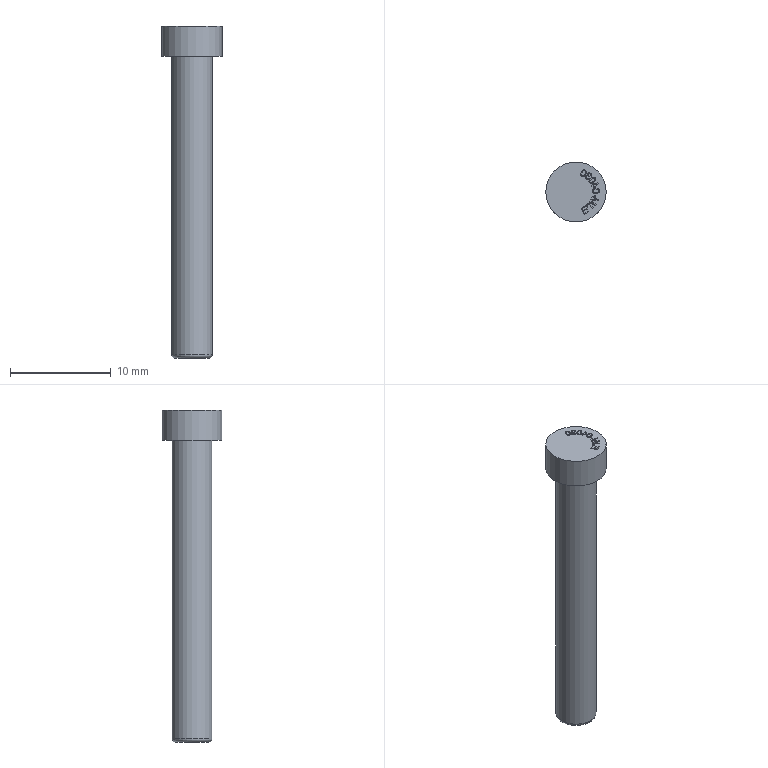Part | NX | features solid 2 | 1 solid | 88 faces | box 6 x 6 x 33 mm | volume 461.337 mm3 | plane 62 | spline 23 | cylinder 2 | torus 1 | commonest cylinder face diameters 4 x1 6 x1